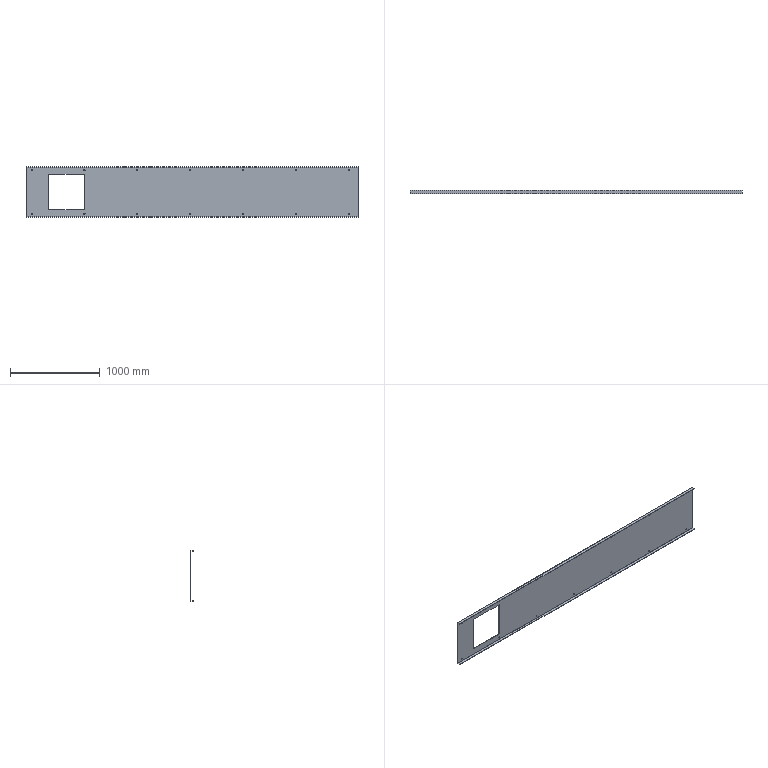Part | STEP file | Input 9 | 1 solid | 46 faces | box 3702 x 35 x 559 mm | volume 9562129 mm3 | cylinder 32 | plane 14 | commonest cylinder face diameters 12 x28 1 x2 10 x2